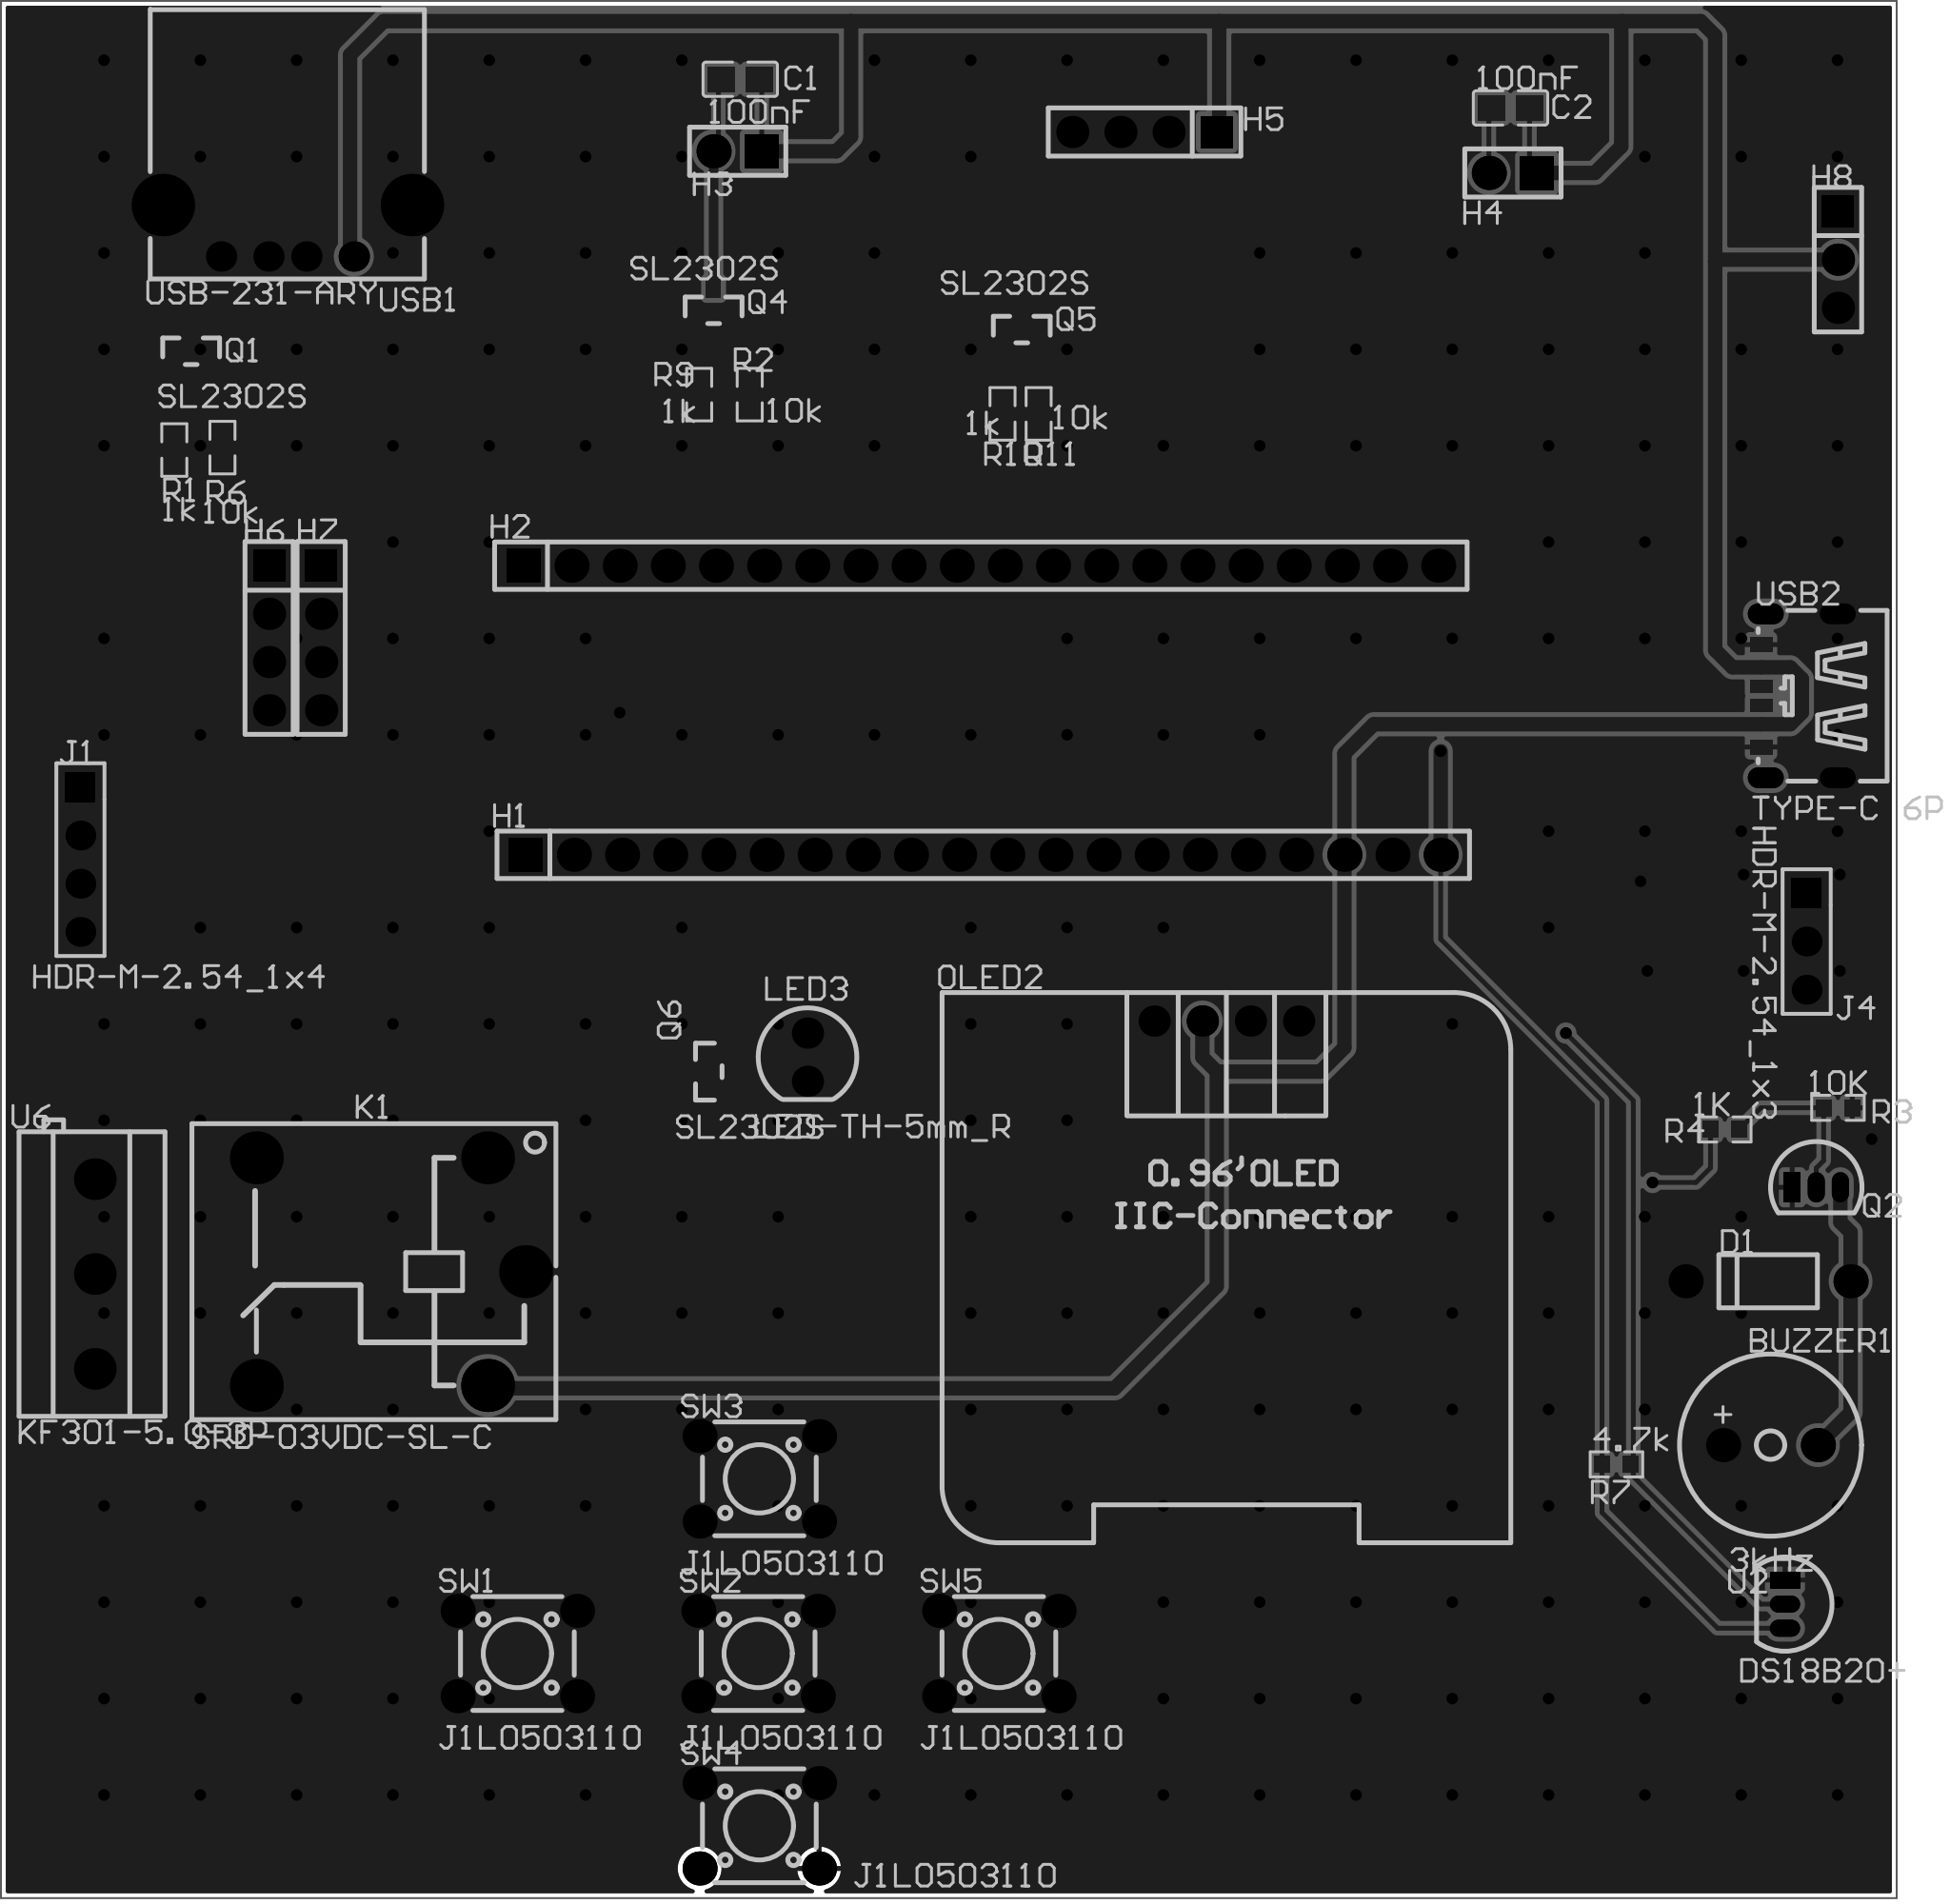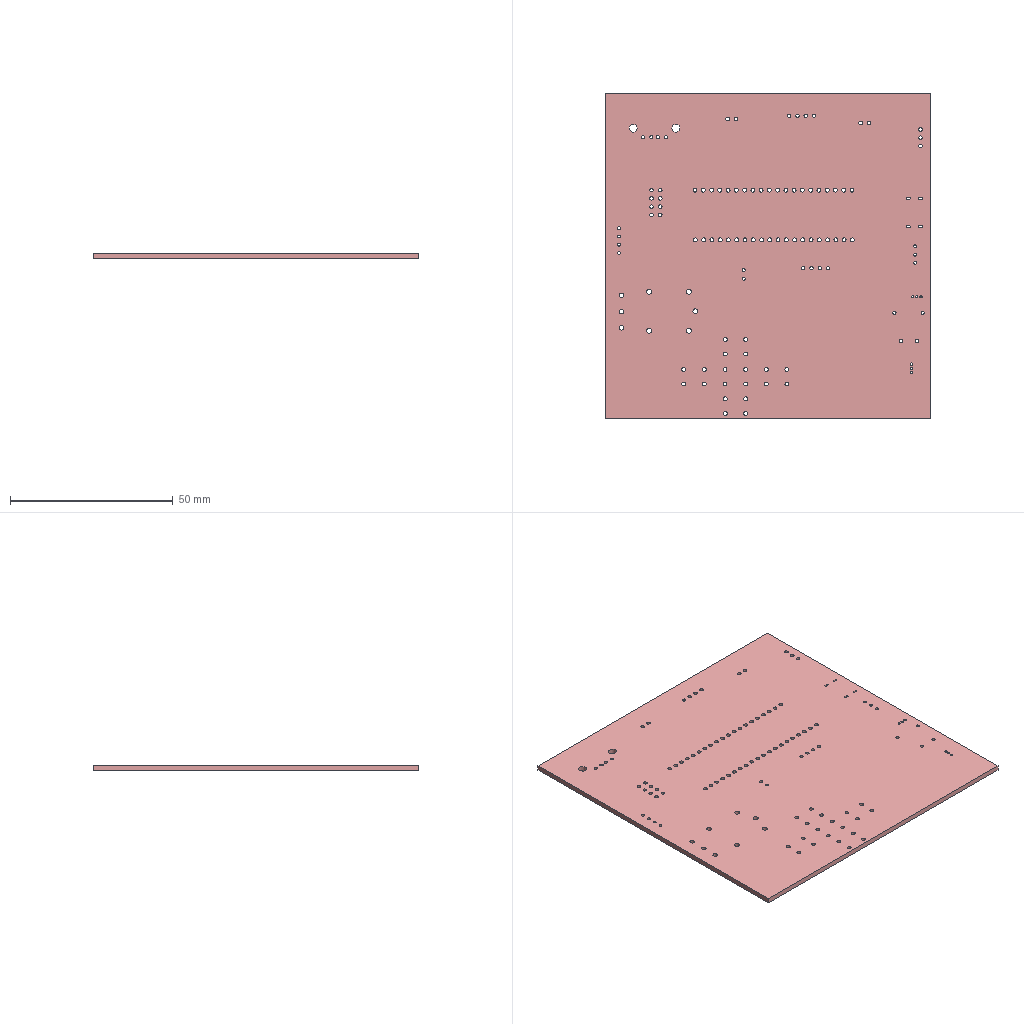Circuit board layout | Altium Designer | box 100 x 100 x 1.6 mm
Layer stack:
# Altium Designer layer stack of  (unit mm; dielectric type: 0 none, 1 core, 2 prepreg, 3 surface material)
index,name,kind,layer,copper_thickness_mm,dielectric_type,dielectric_thickness_mm,dielectric_material,dielectric_constant
0,Top Paste Mask Layer,other,,,,,,
1,Top Silkscreen Layer,other,,,,,,
2,Top Solder Mask Layer,dielectric,,,3,0.01,,3.3
3,Top Layer,copper,Top Layer,0.035,,,,
4,Dielectric1,dielectric,,,3,1.51,FR4,4.5
5,Bottom Layer,copper,Bottom Layer,0.035,,,,
6,Bottom Solder Mask Layer,dielectric,,,3,0.01,,3.3
7,Bottom Silkscreen Layer,other,,,,,,
8,Bottom Paste Mask Layer,other,,,,,,
# drill layer pairs: low layer,high layer
drill_pair,Top Layer,Bottom Layer
Part placement:
Designator,Comment,Layer,Footprint,Center-X(mm),Center-Y(mm),Rotation
BUZZER1,3kHz,TopLayer,BUZ-TH_BD9.6-P5.00-D0.7-FD,181.864,107.188,0
H1,,TopLayer,HDR-TH_20P-P2.54-V-F,140.335,138.303,0
H2,,TopLayer,HDR-TH_20P-P2.54-V-F,140.208,153.543,0
H3,,TopLayer,HDR-TH_2P-P2.54-V-M-1,127.381,175.387,180
H4,,TopLayer,HDR-TH_2P-P2.54-V-M-1,168.275,174.244,180
H5,,TopLayer,HDR-TH_4P-P2.54-V-M,148.844,176.403,180
H6,,TopLayer,HDR-TH_4P-P2.54-V-M,102.663,149.733,270
H7,,TopLayer,HDR-TH_4P-P2.54-V-M,105.41,149.733,270
H8,,TopLayer,HDR-TH_3P-P2.54-V-M,185.42,169.672,270
J1,HDR-M-2.54_1x4,TopLayer,HDR-M-2.54_1X4,92.71,138.049,270
J4,HDR-M-2.54_1x3,TopLayer,HDR-M-2.54_1X3,183.769,133.731,270
K1,SRD-03VDC-SL-C,TopLayer,RELAY-TH_SRD-XXVDC-XL-C,109.093,116.332,180
LED3,LED-TH-5mm_R,TopLayer,LED-TH_BD5.0_RED,131.064,127.635,0
OLED2,,TopLayer,0.96OLED_4P,153.162,129.54,0
Q1,SL2302S,TopLayer,SOT-23_L2.9-W1.3-P1.90-LS2.4-BR,98.552,164.846,270
Q4,SL2302S,TopLayer,SOT-23_L2.9-W1.3-P1.90-LS2.4-BR,126.111,167.005,270
Q5,SL2302S,TopLayer,SOT-23_L2.9-W1.3-P1.90-LS2.4-BR,142.367,165.989,270
Q6,SL2302S,TopLayer,SOT-23_L2.9-W1.3-P1.90-LS2.4-BR,125.857,126.873,0
R1,1k,TopLayer,R0603,97.663,159.639,90
R6,10k,TopLayer,R0603,100.203,159.766,90
R7,4.7k,TopLayer,R0603,173.736,106.172,180
R9,1k,TopLayer,R0603,125.349,162.56,90
R10,1k,TopLayer,R0603,141.351,161.544,90
R11,10k,TopLayer,R0603,143.256,161.544,90
SW1,J1L0503110,TopLayer,SW-TH_4P-L6.0-W6.0-P4.50-LS6.3,115.76,96.203,0
SW2,J1L0503110,TopLayer,SW-TH_4P-L6.0-W6.0-P4.50-LS6.3,128.46,96.203,0
SW3,J1L0503110,TopLayer,SW-TH_4P-L6.0-W6.0-P4.50-LS6.3,128.524,105.41,0
SW4,J1L0503110,TopLayer,SW-TH_4P-L6.0-W6.0-P4.50-LS6.3,128.524,87.122,0
SW5,J1L0503110,TopLayer,SW-TH_4P-L6.0-W6.0-P4.50-LS6.3,141.161,96.203,0
U2,DS18B20+,TopLayer,TO-92-3_L4.9-W3.7-P1.27-L,182.626,98.806,270
U6,KF301-5.0-3P,TopLayer,CONN-TH_3P-P5.00_KF301-5.0-3P,93.472,116.205,90
USB1,USB-231-ARY,TopLayer,USB-A-TH_USB-231-ARY,103.632,171.196,180
USB2,TYPE-C 6P,TopLayer,TYPE-C-SMD_TYPE-C-6P_1,183.388,146.685,90
C1,100nF,TopLayer,C0805,127.516,179.184,180
C2,100nF,TopLayer,C0805,168.148,177.673,180
R2,10k,TopLayer,R0603,128.016,162.56,90
D1,,TopLayer,DO_1N4007,181.737,115.824,0
Q2,,TopLayer,S8050_TO_92,184.277,120.777,0
R3,10K,TopLayer,R0603,185.42,124.968,180
R4,1K,TopLayer,R0603,179.451,123.825,180
Pad and via stacks:
# Altium Designer via and pad stacks of  (unit mm). Each distinct definition once, with the count of objects using it.
# via: kind,start_layer,end_layer,hole_mm,diameter_mm,mode(0 simple;1 top-mid-bottom;2 full stack),diameter_per_layer,count,example_net
# pad: kind,layer,hole_mm,hole_type(0 round;1 square;2 slot),plating,top_size,top_shape(1 round;2 rect;3 octagon;9 rounded rect),mid_size,bottom_size,mode,footprint,size_per_layer,count,example
pad,Multi-Layer,1,0,plated,1.8x1.8,1,1.8x1.8,1.8x1.8,0,BUZ-TH_BD9.6-P5.00-D0.7-FD,,2,BUZZER1.2
pad,Multi-Layer,1.2,0,plated,1.8x1.8,2,1.8x1.8,1.8x1.8,0,HDR-TH_20P-P2.54-V-F,,2,H1.1
pad,Multi-Layer,1.2,0,plated,1.8x1.8,1,1.8x1.8,1.8x1.8,0,HDR-TH_20P-P2.54-V-F,,38,H1.2
pad,Multi-Layer,1.1,0,plated,1.8x1.8,1,1.8x1.8,1.8x1.8,0,HDR-TH_2P-P2.54-V-M-1,,2,H3.2
pad,Multi-Layer,1.1,0,plated,1.8x1.8,2,1.8x1.8,1.8x1.8,0,HDR-TH_2P-P2.54-V-M-1,,2,H3.1
pad,Multi-Layer,1.1,0,plated,1.7x1.7,2,1.7x1.7,1.7x1.7,0,HDR-TH_4P-P2.54-V-M,,3,H5.1
pad,Multi-Layer,1.1,0,plated,1.7x1.7,1,1.7x1.7,1.7x1.7,0,HDR-TH_4P-P2.54-V-M,,9,H5.2
pad,Multi-Layer,1.1,0,plated,1.7x1.7,2,1.7x1.7,1.7x1.7,0,HDR-TH_3P-P2.54-V-M,,1,H8.1
pad,Multi-Layer,1.1,0,plated,1.7x1.7,1,1.7x1.7,1.7x1.7,0,HDR-TH_3P-P2.54-V-M,,2,H8.2
pad,Multi-Layer,0.889,0,plated,1.575x1.575,2,1.575x1.575,1.575x1.575,0,HDR-M-2.54_1X4,,1,J1.1
pad,Multi-Layer,0.889,0,plated,1.575x1.575,1,1.575x1.575,1.575x1.575,0,HDR-M-2.54_1X4,,3,J1.2
pad,Multi-Layer,0.889,0,plated,1.575x1.575,1,1.575x1.575,1.575x1.575,0,HDR-M-2.54_1X3,,2,J4.3
pad,Multi-Layer,0.889,0,plated,1.575x1.575,2,1.575x1.575,1.575x1.575,0,HDR-M-2.54_1X3,,1,J4.1
pad,Multi-Layer,1.524,0,plated,2.794x2.794,1,2.794x2.794,2.794x2.794,0,RELAY-TH_SRD-XXVDC-XL-C,,5,K1.2
pad,Multi-Layer,0.9652,0,plated,1.651x1.651,1,1.651x1.651,1.651x1.651,0,LED-TH_BD5.0_RED,,2,LED3.1
pad,Multi-Layer,1,0,plated,1.65x1.65,1,1.65x1.65,1.65x1.65,0,0.96OLED_4P,,4,OLED2.4
pad,Multi-Layer,1.2,0,plated,1.8x1.8,1,1.8x1.8,1.8x1.8,0,SW-TH_4P-L6.0-W6.0-P4.50-LS6.3,,20,SW1.1
pad,Multi-Layer,0.7,0,plated,0.9x1.6,1,0.9x1.6,0.9x1.6,0,TO-92-3_L4.9-W3.7-P1.27-L,,2,U2.3
pad,Multi-Layer,0.7,0,plated,0.9x1.6,2,0.9x1.6,0.9x1.6,0,TO-92-3_L4.9-W3.7-P1.27-L,,1,U2.1
pad,Multi-Layer,1.4,0,plated,2.2x2.2,1,2.2x2.2,2.2x2.2,0,CONN-TH_3P-P5.00_KF301-5.0-3P,,3,U6.1
pad,Multi-Layer,1,0,plated,1.6x1.6,1,1.6x1.6,1.6x1.6,0,USB-A-TH_USB-231-ARY,,4,USB1.1
pad,Multi-Layer,2.5,0,plated,3.3x3.3,1,3.3x3.3,3.3x3.3,0,USB-A-TH_USB-231-ARY,,2,USB1.5
pad,Multi-Layer,0.6,2,plated,1.1x1.9,1,1.1x1.9,1.1x1.9,0,TYPE-C-SMD_TYPE-C-6P_1,,4,USB2.7
pad,Multi-Layer,1,0,plated,1.8x1.8,1,1.8x1.8,1.8x1.8,0,DO_1N4007,,2,D1.1
pad,Multi-Layer,0.701,0,plated,0.8992x1.6,2,0.8992x1.6,0.8992x1.6,0,S8050_TO_92,,1,Q2.1
pad,Multi-Layer,0.701,0,plated,0.8992x1.6,1,0.8992x1.6,0.8992x1.6,0,S8050_TO_92,,2,Q2.2
pad,Top Layer,0,0,plated,1x0.8,2,1x0.8,1x0.8,0,SOT-23_L2.9-W1.3-P1.90-LS2.4-BR,,12,Q1.2
pad,Top Layer,0,0,plated,0.8065x0.864,2,0.8065x0.864,0.8065x0.864,0,R0603,,18,R1.2
pad,Top Layer,0,0,plated,0.8x1.2,2,0.8x1.2,0.8x1.2,0,TYPE-C-SMD_TYPE-C-6P_1,,2,USB2.B12
pad,Top Layer,0,0,plated,0.7x1.2,2,0.7x1.2,0.7x1.2,0,TYPE-C-SMD_TYPE-C-6P_1,,4,USB2.B9
pad,Top Layer,0,0,plated,1.41x1.35,2,1.41x1.35,1.41x1.35,0,C0805,,4,C1.2
via,Top Layer,Bottom Layer,0.3048,0.61,0,,270,$1N30
Copper pours:
name,layer,net,type(0 solid;1 hatched;2 none)
Top Layer-GND,Top Layer,GND,0
Bottom Layer-GND,Bottom Layer,GND,0